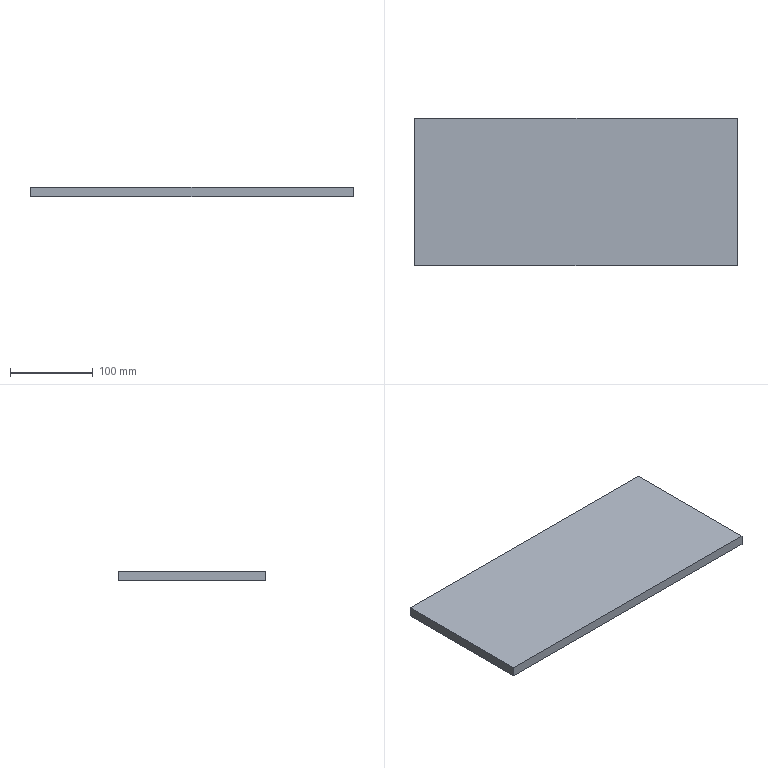Part | SolidWorks | features Extrusion 1 | 1 solid | 6 faces | box 390 x 177.8 x 12 mm | volume 832104 mm3 | plane 6
STEP:
#1=CARTESIAN_POINT('',(-195.,88.9,-6.));
#2=VERTEX_POINT('',#1);
#3=CARTESIAN_POINT('',(-195.,-88.9,-6.));
#4=VERTEX_POINT('',#3);
#5=CARTESIAN_POINT('',(-195.,88.9,-6.));
#6=DIRECTION('',(0.,-1.,0.));
#7=VECTOR('',#6,1000.);
#8=LINE('',#5,#7);
#9=EDGE_CURVE('',#2,#4,#8,.T.);
#10=ORIENTED_EDGE('',*,*,#9,.T.);
#11=CARTESIAN_POINT('',(-195.,-88.9,6.));
#12=VERTEX_POINT('',#11);
#13=CARTESIAN_POINT('',(-195.,-88.9,6.));
#14=DIRECTION('',(0.,0.,-1.));
#15=VECTOR('',#14,1000.);
#16=LINE('',#13,#15);
#17=EDGE_CURVE('',#12,#4,#16,.T.);
#18=ORIENTED_EDGE('',*,*,#17,.F.);
#19=CARTESIAN_POINT('',(-195.,88.9,6.));
#20=VERTEX_POINT('',#19);
#21=CARTESIAN_POINT('',(-195.,88.9,6.));
#22=DIRECTION('',(0.,-1.,0.));
#23=VECTOR('',#22,1000.);
#24=LINE('',#21,#23);
#25=EDGE_CURVE('',#20,#12,#24,.T.);
#26=ORIENTED_EDGE('',*,*,#25,.F.);
#27=CARTESIAN_POINT('',(-195.,88.9,6.));
#28=DIRECTION('',(0.,0.,-1.));
#29=VECTOR('',#28,1000.);
#30=LINE('',#27,#29);
#31=EDGE_CURVE('',#20,#2,#30,.T.);
#32=ORIENTED_EDGE('',*,*,#31,.T.);
#33=EDGE_LOOP('',(#10,#18,#26,#32));
#34=FACE_OUTER_BOUND('',#33,.T.);
#35=CARTESIAN_POINT('',(-195.,88.9,6.));
#36=DIRECTION('',(1.,0.,0.));
#37=DIRECTION('',(0.,0.,-1.));
#38=AXIS2_PLACEMENT_3D('',#35,#36,#37);
#39=PLANE('',#38);
#40=ADVANCED_FACE('',(#34),#39,.F.);
#41=CARTESIAN_POINT('',(195.,-88.9,-6.));
#42=VERTEX_POINT('',#41);
#43=CARTESIAN_POINT('',(-195.,-88.9,-6.));
#44=DIRECTION('',(1.,0.,0.));
#45=VECTOR('',#44,1000.);
#46=LINE('',#43,#45);
#47=EDGE_CURVE('',#4,#42,#46,.T.);
#48=ORIENTED_EDGE('',*,*,#47,.T.);
#49=CARTESIAN_POINT('',(195.,-88.9,6.));
#50=VERTEX_POINT('',#49);
#51=CARTESIAN_POINT('',(195.,-88.9,6.));
#52=DIRECTION('',(0.,0.,-1.));
#53=VECTOR('',#52,1000.);
#54=LINE('',#51,#53);
#55=EDGE_CURVE('',#50,#42,#54,.T.);
#56=ORIENTED_EDGE('',*,*,#55,.F.);
#57=CARTESIAN_POINT('',(-195.,-88.9,6.));
#58=DIRECTION('',(1.,0.,0.));
#59=VECTOR('',#58,1000.);
#60=LINE('',#57,#59);
#61=EDGE_CURVE('',#12,#50,#60,.T.);
#62=ORIENTED_EDGE('',*,*,#61,.F.);
#63=ORIENTED_EDGE('',*,*,#17,.T.);
#64=EDGE_LOOP('',(#48,#56,#62,#63));
#65=FACE_OUTER_BOUND('',#64,.T.);
#66=CARTESIAN_POINT('',(-195.,-88.9,6.));
#67=DIRECTION('',(0.,1.,0.));
#68=DIRECTION('',(-1.,0.,0.));
#69=AXIS2_PLACEMENT_3D('',#66,#67,#68);
#70=PLANE('',#69);
#71=ADVANCED_FACE('',(#65),#70,.F.);
#72=CARTESIAN_POINT('',(195.,88.9,-6.));
#73=VERTEX_POINT('',#72);
#74=CARTESIAN_POINT('',(195.,88.9,-6.));
#75=DIRECTION('',(0.,1.,0.));
#76=VECTOR('',#75,1000.);
#77=LINE('',#74,#76);
#78=EDGE_CURVE('',#42,#73,#77,.T.);
#79=ORIENTED_EDGE('',*,*,#78,.T.);
#80=CARTESIAN_POINT('',(195.,88.9,6.));
#81=VERTEX_POINT('',#80);
#82=CARTESIAN_POINT('',(195.,88.9,6.));
#83=DIRECTION('',(0.,0.,-1.));
#84=VECTOR('',#83,1000.);
#85=LINE('',#82,#84);
#86=EDGE_CURVE('',#81,#73,#85,.T.);
#87=ORIENTED_EDGE('',*,*,#86,.F.);
#88=CARTESIAN_POINT('',(195.,88.9,6.));
#89=DIRECTION('',(0.,1.,0.));
#90=VECTOR('',#89,1000.);
#91=LINE('',#88,#90);
#92=EDGE_CURVE('',#50,#81,#91,.T.);
#93=ORIENTED_EDGE('',*,*,#92,.F.);
#94=ORIENTED_EDGE('',*,*,#55,.T.);
#95=EDGE_LOOP('',(#79,#87,#93,#94));
#96=FACE_OUTER_BOUND('',#95,.T.);
#97=CARTESIAN_POINT('',(195.,88.9,6.));
#98=DIRECTION('',(-1.,0.,0.));
#99=DIRECTION('',(0.,-1.,0.));
#100=AXIS2_PLACEMENT_3D('',#97,#98,#99);
#101=PLANE('',#100);
#102=ADVANCED_FACE('',(#96),#101,.F.);
#103=CARTESIAN_POINT('',(-195.,88.9,-6.));
#104=DIRECTION('',(-1.,0.,0.));
#105=VECTOR('',#104,1000.);
#106=LINE('',#103,#105);
#107=EDGE_CURVE('',#73,#2,#106,.T.);
#108=ORIENTED_EDGE('',*,*,#107,.T.);
#109=ORIENTED_EDGE('',*,*,#31,.F.);
#110=CARTESIAN_POINT('',(-195.,88.9,6.));
#111=DIRECTION('',(-1.,0.,0.));
#112=VECTOR('',#111,1000.);
#113=LINE('',#110,#112);
#114=EDGE_CURVE('',#81,#20,#113,.T.);
#115=ORIENTED_EDGE('',*,*,#114,.F.);
#116=ORIENTED_EDGE('',*,*,#86,.T.);
#117=EDGE_LOOP('',(#108,#109,#115,#116));
#118=FACE_OUTER_BOUND('',#117,.T.);
#119=CARTESIAN_POINT('',(-195.,88.9,6.));
#120=DIRECTION('',(0.,-1.,0.));
#121=DIRECTION('',(1.,0.,0.));
#122=AXIS2_PLACEMENT_3D('',#119,#120,#121);
#123=PLANE('',#122);
#124=ADVANCED_FACE('',(#118),#123,.F.);
#125=ORIENTED_EDGE('',*,*,#25,.T.);
#126=ORIENTED_EDGE('',*,*,#61,.T.);
#127=ORIENTED_EDGE('',*,*,#92,.T.);
#128=ORIENTED_EDGE('',*,*,#114,.T.);
#129=EDGE_LOOP('',(#125,#126,#127,#128));
#130=FACE_OUTER_BOUND('',#129,.T.);
#131=CARTESIAN_POINT('',(-195.,-88.9,6.));
#132=DIRECTION('',(0.,0.,1.));
#133=DIRECTION('',(1.,0.,0.));
#134=AXIS2_PLACEMENT_3D('',#131,#132,#133);
#135=PLANE('',#134);
#136=ADVANCED_FACE('',(#130),#135,.T.);
#137=ORIENTED_EDGE('',*,*,#9,.F.);
#138=ORIENTED_EDGE('',*,*,#107,.F.);
#139=ORIENTED_EDGE('',*,*,#78,.F.);
#140=ORIENTED_EDGE('',*,*,#47,.F.);
#141=EDGE_LOOP('',(#137,#138,#139,#140));
#142=FACE_OUTER_BOUND('',#141,.T.);
#143=CARTESIAN_POINT('',(-195.,-88.9,-6.));
#144=DIRECTION('',(0.,0.,1.));
#145=DIRECTION('',(1.,0.,0.));
#146=AXIS2_PLACEMENT_3D('',#143,#144,#145);
#147=PLANE('',#146);
#148=ADVANCED_FACE('',(#142),#147,.F.);
#149=CLOSED_SHELL('',(#40,#71,#102,#124,#136,#148));
#150=MANIFOLD_SOLID_BREP('',#149);
#151=CARTESIAN_POINT('',(0.,0.,0.));
#152=DIRECTION('',(0.,0.,1.));
#153=DIRECTION('',(1.,0.,0.));
#154=AXIS2_PLACEMENT_3D('',#151,#152,#153);
#155=(LENGTH_UNIT()NAMED_UNIT(*)SI_UNIT(.MILLI.,.METRE.));
#156=UNCERTAINTY_MEASURE_WITH_UNIT(LENGTH_MEASURE(0.00001),#155,'','');
#157=(NAMED_UNIT(*)PLANE_ANGLE_UNIT()SI_UNIT($,.RADIAN.));
#158=(NAMED_UNIT(*)SI_UNIT($,.STERADIAN.)SOLID_ANGLE_UNIT());
#159=(GEOMETRIC_REPRESENTATION_CONTEXT(3)GLOBAL_UNCERTAINTY_ASSIGNED_CONTEXT((#156))GLOBAL_UNIT_ASSIGNED_CONTEXT((#155,#157,#158))REPRESENTATION_CONTEXT('',''));
#160=ADVANCED_BREP_SHAPE_REPRESENTATION('',(#150,#154),#159);